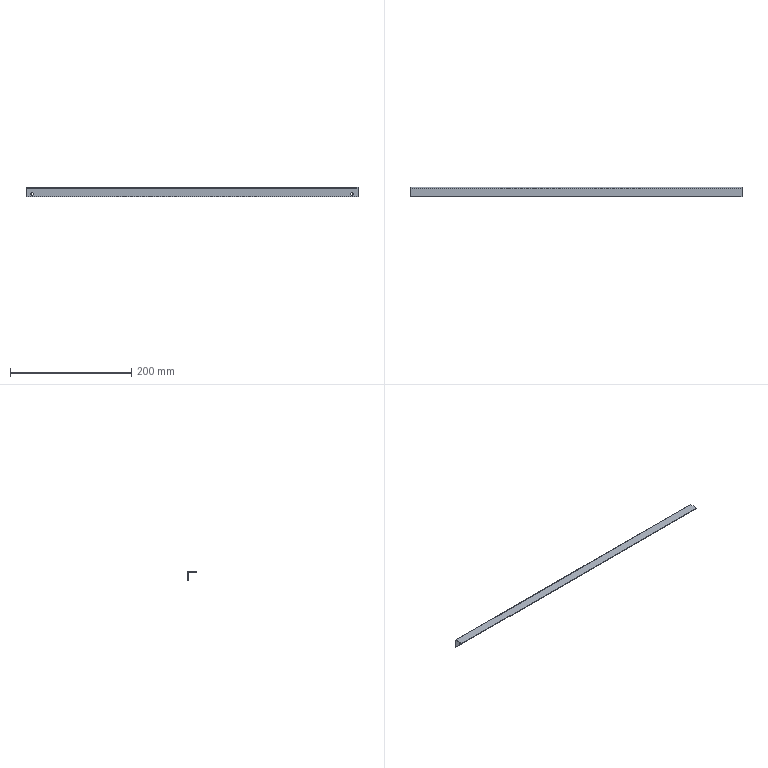Part | SolidWorks | features ICE 1, SplitBody 1 | 1 solid | 18 faces | box 547.1 x 15 x 15 mm | volume 15693 mm3 | plane 12 | cylinder 6 | commonest cylinder face diameters 4.5 x4 0.2 x1 2.2 x1
STEP:
#1=CARTESIAN_POINT('',(541.05,120.,288.));
#2=VERTEX_POINT('',#1);
#3=CARTESIAN_POINT('',(536.55,120.,288.));
#4=VERTEX_POINT('',#3);
#5=CARTESIAN_POINT('',(538.8,120.,288.));
#6=DIRECTION('',(0.,1.,0.));
#7=DIRECTION('',(-1.,0.,0.));
#8=AXIS2_PLACEMENT_3D('',#5,#6,#7);
#9=CIRCLE('',#8,2.25);
#10=EDGE_CURVE('',#2,#4,#9,.T.);
#11=ORIENTED_EDGE('',*,*,#10,.F.);
#12=CARTESIAN_POINT('',(541.05,121.,288.));
#13=VERTEX_POINT('',#12);
#14=CARTESIAN_POINT('',(541.05,111.,288.));
#15=DIRECTION('',(0.,1.,0.));
#16=VECTOR('',#15,1000.);
#17=LINE('',#14,#16);
#18=EDGE_CURVE('',#2,#13,#17,.T.);
#19=ORIENTED_EDGE('',*,*,#18,.T.);
#20=CARTESIAN_POINT('',(536.55,121.,288.));
#21=VERTEX_POINT('',#20);
#22=CARTESIAN_POINT('',(538.8,121.,288.));
#23=DIRECTION('',(0.,1.,0.));
#24=DIRECTION('',(-1.,0.,0.));
#25=AXIS2_PLACEMENT_3D('',#22,#23,#24);
#26=CIRCLE('',#25,2.25);
#27=EDGE_CURVE('',#13,#21,#26,.T.);
#28=ORIENTED_EDGE('',*,*,#27,.T.);
#29=CARTESIAN_POINT('',(536.55,111.,288.));
#30=DIRECTION('',(0.,1.,0.));
#31=VECTOR('',#30,1000.);
#32=LINE('',#29,#31);
#33=EDGE_CURVE('',#4,#21,#32,.T.);
#34=ORIENTED_EDGE('',*,*,#33,.F.);
#35=EDGE_LOOP('',(#11,#19,#28,#34));
#36=FACE_OUTER_BOUND('',#35,.T.);
#37=CARTESIAN_POINT('',(538.8,111.,288.));
#38=DIRECTION('',(0.,1.,0.));
#39=DIRECTION('',(-1.,0.,0.));
#40=AXIS2_PLACEMENT_3D('',#37,#38,#39);
#41=CYLINDRICAL_SURFACE('',#40,2.25);
#42=ADVANCED_FACE('',(#36),#41,.F.);
#43=CARTESIAN_POINT('',(13.95,120.,288.));
#44=VERTEX_POINT('',#43);
#45=CARTESIAN_POINT('',(9.45,120.,288.));
#46=VERTEX_POINT('',#45);
#47=CARTESIAN_POINT('',(11.7,120.,288.));
#48=DIRECTION('',(0.,1.,0.));
#49=DIRECTION('',(-1.,0.,0.));
#50=AXIS2_PLACEMENT_3D('',#47,#48,#49);
#51=CIRCLE('',#50,2.25);
#52=EDGE_CURVE('',#44,#46,#51,.T.);
#53=ORIENTED_EDGE('',*,*,#52,.F.);
#54=CARTESIAN_POINT('',(13.95,121.,288.));
#55=VERTEX_POINT('',#54);
#56=CARTESIAN_POINT('',(13.95,116.,288.));
#57=DIRECTION('',(0.,1.,0.));
#58=VECTOR('',#57,1000.);
#59=LINE('',#56,#58);
#60=EDGE_CURVE('',#44,#55,#59,.T.);
#61=ORIENTED_EDGE('',*,*,#60,.T.);
#62=CARTESIAN_POINT('',(9.45,121.,288.));
#63=VERTEX_POINT('',#62);
#64=CARTESIAN_POINT('',(11.7,121.,288.));
#65=DIRECTION('',(0.,1.,0.));
#66=DIRECTION('',(-1.,0.,0.));
#67=AXIS2_PLACEMENT_3D('',#64,#65,#66);
#68=CIRCLE('',#67,2.25);
#69=EDGE_CURVE('',#55,#63,#68,.T.);
#70=ORIENTED_EDGE('',*,*,#69,.T.);
#71=CARTESIAN_POINT('',(9.45,116.,288.));
#72=DIRECTION('',(0.,1.,0.));
#73=VECTOR('',#72,1000.);
#74=LINE('',#71,#73);
#75=EDGE_CURVE('',#46,#63,#74,.T.);
#76=ORIENTED_EDGE('',*,*,#75,.F.);
#77=EDGE_LOOP('',(#53,#61,#70,#76));
#78=FACE_OUTER_BOUND('',#77,.T.);
#79=CARTESIAN_POINT('',(11.7,116.,288.));
#80=DIRECTION('',(0.,1.,0.));
#81=DIRECTION('',(-1.,0.,0.));
#82=AXIS2_PLACEMENT_3D('',#79,#80,#81);
#83=CYLINDRICAL_SURFACE('',#82,2.25);
#84=ADVANCED_FACE('',(#78),#83,.F.);
#85=CARTESIAN_POINT('',(1.7,121.,297.7));
#86=VERTEX_POINT('',#85);
#87=CARTESIAN_POINT('',(1.7,120.,297.7));
#88=VERTEX_POINT('',#87);
#89=CARTESIAN_POINT('',(1.7,121.,297.7));
#90=DIRECTION('',(0.,-1.,0.));
#91=VECTOR('',#90,1000.);
#92=LINE('',#89,#91);
#93=EDGE_CURVE('',#86,#88,#92,.T.);
#94=ORIENTED_EDGE('',*,*,#93,.T.);
#95=CARTESIAN_POINT('',(1.7,119.9,297.8));
#96=VERTEX_POINT('',#95);
#97=CARTESIAN_POINT('',(1.7,119.9,297.7));
#98=DIRECTION('',(1.,0.,0.));
#99=DIRECTION('',(0.,0.,-1.));
#100=AXIS2_PLACEMENT_3D('',#97,#98,#99);
#101=CIRCLE('',#100,0.1);
#102=EDGE_CURVE('',#88,#96,#101,.T.);
#103=ORIENTED_EDGE('',*,*,#102,.T.);
#104=CARTESIAN_POINT('',(1.7,119.9,298.8));
#105=VERTEX_POINT('',#104);
#106=CARTESIAN_POINT('',(1.7,119.9,297.8));
#107=DIRECTION('',(0.,0.,1.));
#108=VECTOR('',#107,1000.);
#109=LINE('',#106,#108);
#110=EDGE_CURVE('',#96,#105,#109,.T.);
#111=ORIENTED_EDGE('',*,*,#110,.T.);
#112=CARTESIAN_POINT('',(1.7,119.9,297.7));
#113=DIRECTION('',(1.,0.,0.));
#114=DIRECTION('',(0.,-1.,0.));
#115=AXIS2_PLACEMENT_3D('',#112,#113,#114);
#116=CIRCLE('',#115,1.1);
#117=EDGE_CURVE('',#86,#105,#116,.T.);
#118=ORIENTED_EDGE('',*,*,#117,.F.);
#119=EDGE_LOOP('',(#94,#103,#111,#118));
#120=FACE_OUTER_BOUND('',#119,.T.);
#121=CARTESIAN_POINT('',(1.7,121.,297.7));
#122=DIRECTION('',(-1.,0.,0.));
#123=DIRECTION('',(0.,1.,0.));
#124=AXIS2_PLACEMENT_3D('',#121,#122,#123);
#125=PLANE('',#124);
#126=ADVANCED_FACE('',(#120),#125,.T.);
#127=CARTESIAN_POINT('',(1.7,121.,283.8));
#128=VERTEX_POINT('',#127);
#129=CARTESIAN_POINT('',(1.7,121.,283.8));
#130=DIRECTION('',(0.,0.,1.));
#131=VECTOR('',#130,1000.);
#132=LINE('',#129,#131);
#133=EDGE_CURVE('',#128,#86,#132,.T.);
#134=ORIENTED_EDGE('',*,*,#133,.F.);
#135=CARTESIAN_POINT('',(1.7,120.,283.8));
#136=VERTEX_POINT('',#135);
#137=CARTESIAN_POINT('',(1.7,120.,283.8));
#138=DIRECTION('',(0.,1.,0.));
#139=VECTOR('',#138,1000.);
#140=LINE('',#137,#139);
#141=EDGE_CURVE('',#136,#128,#140,.T.);
#142=ORIENTED_EDGE('',*,*,#141,.F.);
#143=CARTESIAN_POINT('',(1.7,120.,283.8));
#144=DIRECTION('',(0.,0.,1.));
#145=VECTOR('',#144,1000.);
#146=LINE('',#143,#145);
#147=EDGE_CURVE('',#136,#88,#146,.T.);
#148=ORIENTED_EDGE('',*,*,#147,.T.);
#149=ORIENTED_EDGE('',*,*,#93,.F.);
#150=EDGE_LOOP('',(#134,#142,#148,#149));
#151=FACE_OUTER_BOUND('',#150,.T.);
#152=CARTESIAN_POINT('',(1.7,119.9,297.8));
#153=DIRECTION('',(-1.,0.,0.));
#154=DIRECTION('',(0.,1.,0.));
#155=AXIS2_PLACEMENT_3D('',#152,#153,#154);
#156=PLANE('',#155);
#157=ADVANCED_FACE('',(#151),#156,.T.);
#158=CARTESIAN_POINT('',(548.8,119.9,297.8));
#159=VERTEX_POINT('',#158);
#160=CARTESIAN_POINT('',(548.8,106.,297.8));
#161=VERTEX_POINT('',#160);
#162=CARTESIAN_POINT('',(548.8,121.,297.8));
#163=DIRECTION('',(0.,-1.,0.));
#164=VECTOR('',#163,1000.);
#165=LINE('',#162,#164);
#166=EDGE_CURVE('',#159,#161,#165,.T.);
#167=ORIENTED_EDGE('',*,*,#166,.T.);
#168=CARTESIAN_POINT('',(1.7,106.,297.8));
#169=VERTEX_POINT('',#168);
#170=CARTESIAN_POINT('',(570.013,106.,297.8));
#171=DIRECTION('',(-1.,0.,0.));
#172=VECTOR('',#171,1000.);
#173=LINE('',#170,#172);
#174=EDGE_CURVE('',#161,#169,#173,.T.);
#175=ORIENTED_EDGE('',*,*,#174,.T.);
#176=CARTESIAN_POINT('',(1.7,121.,297.8));
#177=DIRECTION('',(0.,-1.,0.));
#178=VECTOR('',#177,1000.);
#179=LINE('',#176,#178);
#180=EDGE_CURVE('',#96,#169,#179,.T.);
#181=ORIENTED_EDGE('',*,*,#180,.F.);
#182=CARTESIAN_POINT('',(570.013,119.9,297.8));
#183=DIRECTION('',(-1.,0.,0.));
#184=VECTOR('',#183,1000.);
#185=LINE('',#182,#184);
#186=EDGE_CURVE('',#159,#96,#185,.T.);
#187=ORIENTED_EDGE('',*,*,#186,.F.);
#188=EDGE_LOOP('',(#167,#175,#181,#187));
#189=FACE_OUTER_BOUND('',#188,.T.);
#190=CARTESIAN_POINT('',(570.013,121.,297.8));
#191=DIRECTION('',(0.,0.,1.));
#192=DIRECTION('',(1.,0.,0.));
#193=AXIS2_PLACEMENT_3D('',#190,#191,#192);
#194=PLANE('',#193);
#195=ADVANCED_FACE('',(#189),#194,.F.);
#196=CARTESIAN_POINT('',(548.8,106.,298.8));
#197=VERTEX_POINT('',#196);
#198=CARTESIAN_POINT('',(1.7,106.,298.8));
#199=VERTEX_POINT('',#198);
#200=CARTESIAN_POINT('',(570.013,106.,298.8));
#201=DIRECTION('',(-1.,0.,0.));
#202=VECTOR('',#201,1000.);
#203=LINE('',#200,#202);
#204=EDGE_CURVE('',#197,#199,#203,.T.);
#205=ORIENTED_EDGE('',*,*,#204,.T.);
#206=CARTESIAN_POINT('',(1.7,106.,298.8));
#207=DIRECTION('',(0.,0.,-1.));
#208=VECTOR('',#207,1000.);
#209=LINE('',#206,#208);
#210=EDGE_CURVE('',#199,#169,#209,.T.);
#211=ORIENTED_EDGE('',*,*,#210,.T.);
#212=ORIENTED_EDGE('',*,*,#174,.F.);
#213=CARTESIAN_POINT('',(548.8,106.,298.8));
#214=DIRECTION('',(0.,0.,-1.));
#215=VECTOR('',#214,1000.);
#216=LINE('',#213,#215);
#217=EDGE_CURVE('',#197,#161,#216,.T.);
#218=ORIENTED_EDGE('',*,*,#217,.F.);
#219=EDGE_LOOP('',(#205,#211,#212,#218));
#220=FACE_OUTER_BOUND('',#219,.T.);
#221=CARTESIAN_POINT('',(570.013,106.,298.8));
#222=DIRECTION('',(0.,-1.,0.));
#223=DIRECTION('',(-1.,0.,0.));
#224=AXIS2_PLACEMENT_3D('',#221,#222,#223);
#225=PLANE('',#224);
#226=ADVANCED_FACE('',(#220),#225,.T.);
#227=CARTESIAN_POINT('',(548.8,119.9,298.8));
#228=VERTEX_POINT('',#227);
#229=CARTESIAN_POINT('',(570.013,119.9,298.8));
#230=DIRECTION('',(-1.,0.,0.));
#231=VECTOR('',#230,1000.);
#232=LINE('',#229,#231);
#233=EDGE_CURVE('',#228,#105,#232,.T.);
#234=ORIENTED_EDGE('',*,*,#233,.T.);
#235=CARTESIAN_POINT('',(1.7,121.,298.8));
#236=DIRECTION('',(0.,-1.,0.));
#237=VECTOR('',#236,1000.);
#238=LINE('',#235,#237);
#239=EDGE_CURVE('',#105,#199,#238,.T.);
#240=ORIENTED_EDGE('',*,*,#239,.T.);
#241=ORIENTED_EDGE('',*,*,#204,.F.);
#242=CARTESIAN_POINT('',(548.8,121.,298.8));
#243=DIRECTION('',(0.,-1.,0.));
#244=VECTOR('',#243,1000.);
#245=LINE('',#242,#244);
#246=EDGE_CURVE('',#228,#197,#245,.T.);
#247=ORIENTED_EDGE('',*,*,#246,.F.);
#248=EDGE_LOOP('',(#234,#240,#241,#247));
#249=FACE_OUTER_BOUND('',#248,.T.);
#250=CARTESIAN_POINT('',(570.013,121.,298.8));
#251=DIRECTION('',(0.,0.,1.));
#252=DIRECTION('',(1.,0.,0.));
#253=AXIS2_PLACEMENT_3D('',#250,#251,#252);
#254=PLANE('',#253);
#255=ADVANCED_FACE('',(#249),#254,.T.);
#256=CARTESIAN_POINT('',(548.8,121.,297.7));
#257=VERTEX_POINT('',#256);
#258=CARTESIAN_POINT('',(570.013,121.,297.7));
#259=DIRECTION('',(-1.,0.,0.));
#260=VECTOR('',#259,1000.);
#261=LINE('',#258,#260);
#262=EDGE_CURVE('',#257,#86,#261,.T.);
#263=ORIENTED_EDGE('',*,*,#262,.T.);
#264=ORIENTED_EDGE('',*,*,#117,.T.);
#265=ORIENTED_EDGE('',*,*,#233,.F.);
#266=CARTESIAN_POINT('',(548.8,119.9,297.7));
#267=DIRECTION('',(-1.,0.,0.));
#268=DIRECTION('',(0.,1.,0.));
#269=AXIS2_PLACEMENT_3D('',#266,#267,#268);
#270=CIRCLE('',#269,1.1);
#271=EDGE_CURVE('',#228,#257,#270,.T.);
#272=ORIENTED_EDGE('',*,*,#271,.T.);
#273=EDGE_LOOP('',(#263,#264,#265,#272));
#274=FACE_OUTER_BOUND('',#273,.T.);
#275=CARTESIAN_POINT('',(570.013,119.9,297.7));
#276=DIRECTION('',(-1.,0.,0.));
#277=DIRECTION('',(0.,1.,0.));
#278=AXIS2_PLACEMENT_3D('',#275,#276,#277);
#279=CYLINDRICAL_SURFACE('',#278,1.1);
#280=ADVANCED_FACE('',(#274),#279,.T.);
#281=CARTESIAN_POINT('',(538.8,121.,288.));
#282=DIRECTION('',(0.,1.,0.));
#283=DIRECTION('',(-1.,0.,0.));
#284=AXIS2_PLACEMENT_3D('',#281,#282,#283);
#285=CIRCLE('',#284,2.25);
#286=EDGE_CURVE('',#21,#13,#285,.T.);
#287=ORIENTED_EDGE('',*,*,#286,.F.);
#288=ORIENTED_EDGE('',*,*,#27,.F.);
#289=EDGE_LOOP('',(#287,#288));
#290=FACE_BOUND('',#289,.T.);
#291=CARTESIAN_POINT('',(11.7,121.,288.));
#292=DIRECTION('',(0.,1.,0.));
#293=DIRECTION('',(-1.,0.,0.));
#294=AXIS2_PLACEMENT_3D('',#291,#292,#293);
#295=CIRCLE('',#294,2.25);
#296=EDGE_CURVE('',#63,#55,#295,.T.);
#297=ORIENTED_EDGE('',*,*,#296,.F.);
#298=ORIENTED_EDGE('',*,*,#69,.F.);
#299=EDGE_LOOP('',(#297,#298));
#300=FACE_BOUND('',#299,.T.);
#301=CARTESIAN_POINT('',(548.8,121.,283.8));
#302=VERTEX_POINT('',#301);
#303=CARTESIAN_POINT('',(570.013,121.,283.8));
#304=DIRECTION('',(-1.,0.,0.));
#305=VECTOR('',#304,1000.);
#306=LINE('',#303,#305);
#307=EDGE_CURVE('',#302,#128,#306,.T.);
#308=ORIENTED_EDGE('',*,*,#307,.T.);
#309=ORIENTED_EDGE('',*,*,#133,.T.);
#310=ORIENTED_EDGE('',*,*,#262,.F.);
#311=CARTESIAN_POINT('',(548.8,121.,283.8));
#312=DIRECTION('',(0.,0.,1.));
#313=VECTOR('',#312,1000.);
#314=LINE('',#311,#313);
#315=EDGE_CURVE('',#302,#257,#314,.T.);
#316=ORIENTED_EDGE('',*,*,#315,.F.);
#317=EDGE_LOOP('',(#308,#309,#310,#316));
#318=FACE_OUTER_BOUND('',#317,.T.);
#319=CARTESIAN_POINT('',(570.013,121.,283.8));
#320=DIRECTION('',(0.,1.,0.));
#321=DIRECTION('',(1.,0.,0.));
#322=AXIS2_PLACEMENT_3D('',#319,#320,#321);
#323=PLANE('',#322);
#324=ADVANCED_FACE('',(#290,#300,#318),#323,.T.);
#325=CARTESIAN_POINT('',(548.8,120.,283.8));
#326=VERTEX_POINT('',#325);
#327=CARTESIAN_POINT('',(570.013,120.,283.8));
#328=DIRECTION('',(-1.,0.,0.));
#329=VECTOR('',#328,1000.);
#330=LINE('',#327,#329);
#331=EDGE_CURVE('',#326,#136,#330,.T.);
#332=ORIENTED_EDGE('',*,*,#331,.T.);
#333=ORIENTED_EDGE('',*,*,#141,.T.);
#334=ORIENTED_EDGE('',*,*,#307,.F.);
#335=CARTESIAN_POINT('',(548.8,120.,283.8));
#336=DIRECTION('',(0.,1.,0.));
#337=VECTOR('',#336,1000.);
#338=LINE('',#335,#337);
#339=EDGE_CURVE('',#326,#302,#338,.T.);
#340=ORIENTED_EDGE('',*,*,#339,.F.);
#341=EDGE_LOOP('',(#332,#333,#334,#340));
#342=FACE_OUTER_BOUND('',#341,.T.);
#343=CARTESIAN_POINT('',(570.013,120.,283.8));
#344=DIRECTION('',(0.,0.,-1.));
#345=DIRECTION('',(-1.,0.,0.));
#346=AXIS2_PLACEMENT_3D('',#343,#344,#345);
#347=PLANE('',#346);
#348=ADVANCED_FACE('',(#342),#347,.T.);
#349=CARTESIAN_POINT('',(538.8,120.,288.));
#350=DIRECTION('',(0.,1.,0.));
#351=DIRECTION('',(-1.,0.,0.));
#352=AXIS2_PLACEMENT_3D('',#349,#350,#351);
#353=CIRCLE('',#352,2.25);
#354=EDGE_CURVE('',#4,#2,#353,.T.);
#355=ORIENTED_EDGE('',*,*,#354,.T.);
#356=ORIENTED_EDGE('',*,*,#10,.T.);
#357=EDGE_LOOP('',(#355,#356));
#358=FACE_BOUND('',#357,.T.);
#359=CARTESIAN_POINT('',(11.7,120.,288.));
#360=DIRECTION('',(0.,1.,0.));
#361=DIRECTION('',(-1.,0.,0.));
#362=AXIS2_PLACEMENT_3D('',#359,#360,#361);
#363=CIRCLE('',#362,2.25);
#364=EDGE_CURVE('',#46,#44,#363,.T.);
#365=ORIENTED_EDGE('',*,*,#364,.T.);
#366=ORIENTED_EDGE('',*,*,#52,.T.);
#367=EDGE_LOOP('',(#365,#366));
#368=FACE_BOUND('',#367,.T.);
#369=CARTESIAN_POINT('',(548.8,120.,297.7));
#370=VERTEX_POINT('',#369);
#371=CARTESIAN_POINT('',(548.8,120.,283.8));
#372=DIRECTION('',(0.,0.,1.));
#373=VECTOR('',#372,1000.);
#374=LINE('',#371,#373);
#375=EDGE_CURVE('',#326,#370,#374,.T.);
#376=ORIENTED_EDGE('',*,*,#375,.T.);
#377=CARTESIAN_POINT('',(570.013,120.,297.7));
#378=DIRECTION('',(-1.,0.,0.));
#379=VECTOR('',#378,1000.);
#380=LINE('',#377,#379);
#381=EDGE_CURVE('',#370,#88,#380,.T.);
#382=ORIENTED_EDGE('',*,*,#381,.T.);
#383=ORIENTED_EDGE('',*,*,#147,.F.);
#384=ORIENTED_EDGE('',*,*,#331,.F.);
#385=EDGE_LOOP('',(#376,#382,#383,#384));
#386=FACE_OUTER_BOUND('',#385,.T.);
#387=CARTESIAN_POINT('',(570.013,120.,283.8));
#388=DIRECTION('',(0.,1.,0.));
#389=DIRECTION('',(1.,0.,0.));
#390=AXIS2_PLACEMENT_3D('',#387,#388,#389);
#391=PLANE('',#390);
#392=ADVANCED_FACE('',(#358,#368,#386),#391,.F.);
#393=CARTESIAN_POINT('',(548.8,119.9,297.7));
#394=DIRECTION('',(1.,0.,0.));
#395=DIRECTION('',(0.,-1.,0.));
#396=AXIS2_PLACEMENT_3D('',#393,#394,#395);
#397=CIRCLE('',#396,0.1);
#398=EDGE_CURVE('',#370,#159,#397,.T.);
#399=ORIENTED_EDGE('',*,*,#398,.T.);
#400=ORIENTED_EDGE('',*,*,#186,.T.);
#401=ORIENTED_EDGE('',*,*,#102,.F.);
#402=ORIENTED_EDGE('',*,*,#381,.F.);
#403=EDGE_LOOP('',(#399,#400,#401,#402));
#404=FACE_OUTER_BOUND('',#403,.T.);
#405=CARTESIAN_POINT('',(570.013,119.9,297.7));
#406=DIRECTION('',(-1.,0.,0.));
#407=DIRECTION('',(0.,1.,0.));
#408=AXIS2_PLACEMENT_3D('',#405,#406,#407);
#409=CYLINDRICAL_SURFACE('',#408,0.1);
#410=ADVANCED_FACE('',(#404),#409,.F.);
#411=ORIENTED_EDGE('',*,*,#180,.T.);
#412=ORIENTED_EDGE('',*,*,#210,.F.);
#413=ORIENTED_EDGE('',*,*,#239,.F.);
#414=ORIENTED_EDGE('',*,*,#110,.F.);
#415=EDGE_LOOP('',(#411,#412,#413,#414));
#416=FACE_OUTER_BOUND('',#415,.T.);
#417=CARTESIAN_POINT('',(1.7,119.9,297.7));
#418=DIRECTION('',(1.,0.,0.));
#419=DIRECTION('',(0.,1.,0.));
#420=AXIS2_PLACEMENT_3D('',#417,#418,#419);
#421=PLANE('',#420);
#422=ADVANCED_FACE('',(#416),#421,.F.);
#423=ORIENTED_EDGE('',*,*,#375,.F.);
#424=ORIENTED_EDGE('',*,*,#339,.T.);
#425=ORIENTED_EDGE('',*,*,#315,.T.);
#426=CARTESIAN_POINT('',(548.8,120.,297.7));
#427=DIRECTION('',(0.,1.,0.));
#428=VECTOR('',#427,1000.);
#429=LINE('',#426,#428);
#430=EDGE_CURVE('',#370,#257,#429,.T.);
#431=ORIENTED_EDGE('',*,*,#430,.F.);
#432=EDGE_LOOP('',(#423,#424,#425,#431));
#433=FACE_OUTER_BOUND('',#432,.T.);
#434=CARTESIAN_POINT('',(548.8,120.,283.8));
#435=DIRECTION('',(1.,0.,0.));
#436=DIRECTION('',(0.,0.,1.));
#437=AXIS2_PLACEMENT_3D('',#434,#435,#436);
#438=PLANE('',#437);
#439=ADVANCED_FACE('',(#433),#438,.T.);
#440=ORIENTED_EDGE('',*,*,#217,.T.);
#441=ORIENTED_EDGE('',*,*,#166,.F.);
#442=CARTESIAN_POINT('',(548.8,119.9,298.8));
#443=DIRECTION('',(0.,0.,-1.));
#444=VECTOR('',#443,1000.);
#445=LINE('',#442,#444);
#446=EDGE_CURVE('',#228,#159,#445,.T.);
#447=ORIENTED_EDGE('',*,*,#446,.F.);
#448=ORIENTED_EDGE('',*,*,#246,.T.);
#449=EDGE_LOOP('',(#440,#441,#447,#448));
#450=FACE_OUTER_BOUND('',#449,.T.);
#451=CARTESIAN_POINT('',(548.8,121.,298.8));
#452=DIRECTION('',(1.,0.,0.));
#453=DIRECTION('',(0.,-1.,0.));
#454=AXIS2_PLACEMENT_3D('',#451,#452,#453);
#455=PLANE('',#454);
#456=ADVANCED_FACE('',(#450),#455,.T.);
#457=ORIENTED_EDGE('',*,*,#271,.F.);
#458=ORIENTED_EDGE('',*,*,#446,.T.);
#459=ORIENTED_EDGE('',*,*,#398,.F.);
#460=ORIENTED_EDGE('',*,*,#430,.T.);
#461=EDGE_LOOP('',(#457,#458,#459,#460));
#462=FACE_OUTER_BOUND('',#461,.T.);
#463=CARTESIAN_POINT('',(548.8,119.9,297.7));
#464=DIRECTION('',(-1.,0.,0.));
#465=DIRECTION('',(0.,1.,0.));
#466=AXIS2_PLACEMENT_3D('',#463,#464,#465);
#467=PLANE('',#466);
#468=ADVANCED_FACE('',(#462),#467,.F.);
#469=ORIENTED_EDGE('',*,*,#60,.F.);
#470=ORIENTED_EDGE('',*,*,#364,.F.);
#471=ORIENTED_EDGE('',*,*,#75,.T.);
#472=ORIENTED_EDGE('',*,*,#296,.T.);
#473=EDGE_LOOP('',(#469,#470,#471,#472));
#474=FACE_OUTER_BOUND('',#473,.T.);
#475=CARTESIAN_POINT('',(11.7,116.,288.));
#476=DIRECTION('',(0.,1.,0.));
#477=DIRECTION('',(-1.,0.,0.));
#478=AXIS2_PLACEMENT_3D('',#475,#476,#477);
#479=CYLINDRICAL_SURFACE('',#478,2.25);
#480=ADVANCED_FACE('',(#474),#479,.F.);
#481=ORIENTED_EDGE('',*,*,#18,.F.);
#482=ORIENTED_EDGE('',*,*,#354,.F.);
#483=ORIENTED_EDGE('',*,*,#33,.T.);
#484=ORIENTED_EDGE('',*,*,#286,.T.);
#485=EDGE_LOOP('',(#481,#482,#483,#484));
#486=FACE_OUTER_BOUND('',#485,.T.);
#487=CARTESIAN_POINT('',(538.8,111.,288.));
#488=DIRECTION('',(0.,1.,0.));
#489=DIRECTION('',(-1.,0.,0.));
#490=AXIS2_PLACEMENT_3D('',#487,#488,#489);
#491=CYLINDRICAL_SURFACE('',#490,2.25);
#492=ADVANCED_FACE('',(#486),#491,.F.);
#493=CLOSED_SHELL('',(#42,#84,#126,#157,#195,#226,#255,#280,#324,#348,#392,#410,#422,#439,#456,#468,#480,#492));
#494=MANIFOLD_SOLID_BREP('',#493);
#495=CARTESIAN_POINT('',(0.,0.,0.));
#496=DIRECTION('',(0.,0.,1.));
#497=DIRECTION('',(1.,0.,0.));
#498=AXIS2_PLACEMENT_3D('',#495,#496,#497);
#499=(LENGTH_UNIT()NAMED_UNIT(*)SI_UNIT(.MILLI.,.METRE.));
#500=UNCERTAINTY_MEASURE_WITH_UNIT(LENGTH_MEASURE(0.00001),#499,'','');
#501=(NAMED_UNIT(*)PLANE_ANGLE_UNIT()SI_UNIT($,.RADIAN.));
#502=(NAMED_UNIT(*)SI_UNIT($,.STERADIAN.)SOLID_ANGLE_UNIT());
#503=(GEOMETRIC_REPRESENTATION_CONTEXT(3)GLOBAL_UNCERTAINTY_ASSIGNED_CONTEXT((#500))GLOBAL_UNIT_ASSIGNED_CONTEXT((#499,#501,#502))REPRESENTATION_CONTEXT('',''));
#504=ADVANCED_BREP_SHAPE_REPRESENTATION('',(#494,#498),#503);